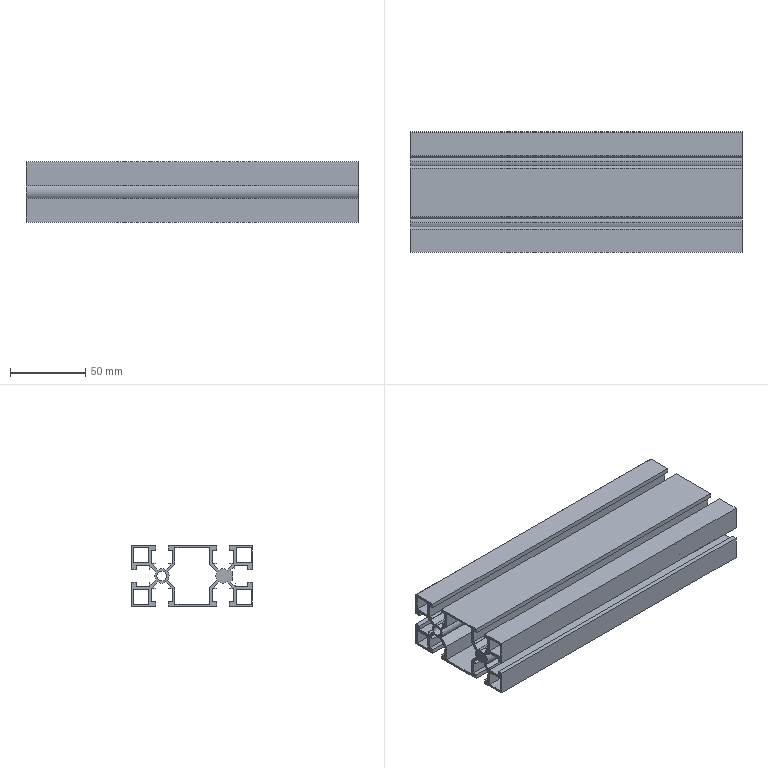Part | SolidWorks | features WeldMemberFeat 1, WeldmentFeature 1 | 1 solid | 124 faces | box 220 x 80 x 40 mm | volume 163035 mm3 | plane 110 | cylinder 14 | commonest cylinder face diameters 9.6 x9 0.6 x2 6.6 x2 13.3 x1